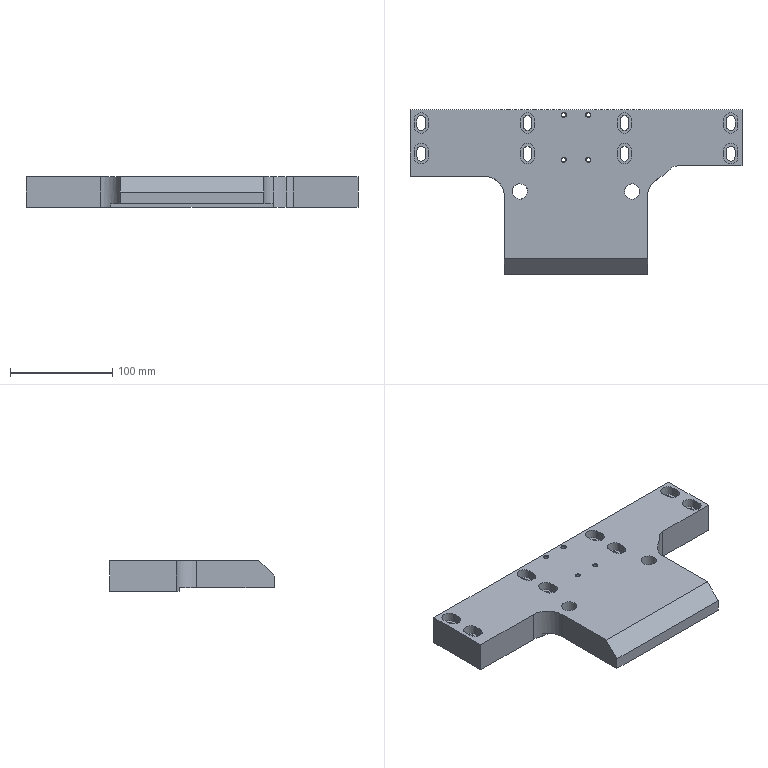Part | STEP file | Tube feed_id886_x_t | 1 solid | 103 faces | box 325 x 161 x 30 mm | volume 914325 mm3 | plane 53 | cylinder 42 | cone 8 | commonest cylinder face diameters 8.5 x16 14 x16 4.2 x4 15 x2 40 x2 20 x1